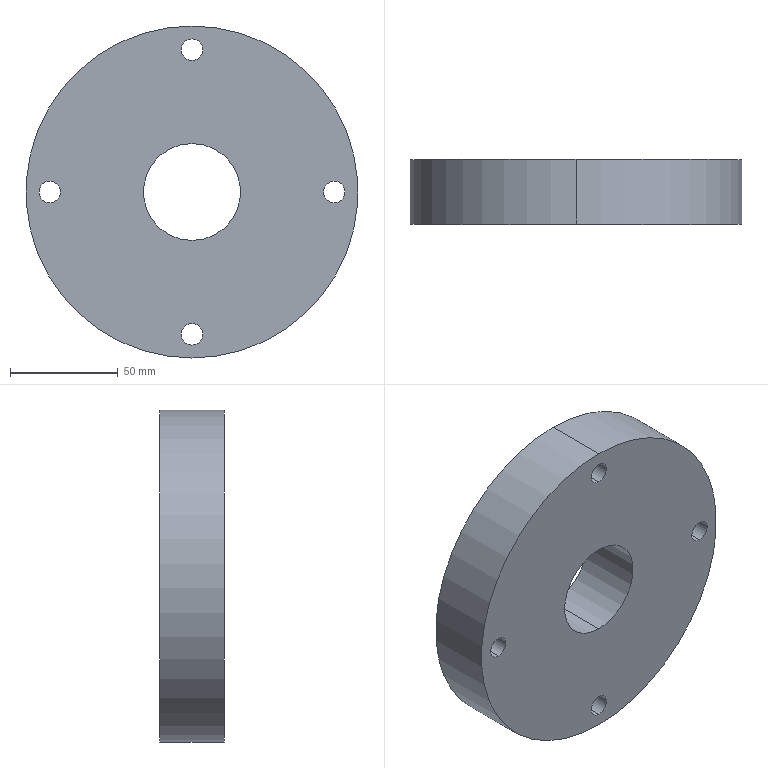Part | SolidWorks | features BaseBody 1 | 1 solid | 14 faces | box 154 x 30 x 154 mm | volume 501657 mm3 | cylinder 12 | plane 2 | commonest cylinder face diameters 10 x8 45 x2 154 x2
STEP:
#1=CARTESIAN_POINT('',(0.,30.,22.5));
#2=VERTEX_POINT('',#1);
#3=CARTESIAN_POINT('',(0.,30.,-22.5));
#4=VERTEX_POINT('',#3);
#5=CARTESIAN_POINT('',(0.,30.,0.));
#6=DIRECTION('',(0.,-1.,0.));
#7=DIRECTION('',(0.,0.,-1.));
#8=AXIS2_PLACEMENT_3D('',#5,#6,#7);
#9=CIRCLE('',#8,22.5);
#10=EDGE_CURVE('',#2,#4,#9,.T.);
#11=ORIENTED_EDGE('',*,*,#10,.F.);
#12=CARTESIAN_POINT('',(0.,0.,22.5));
#13=VERTEX_POINT('',#12);
#14=CARTESIAN_POINT('',(0.,30.,22.5));
#15=DIRECTION('',(0.,-1.,0.));
#16=VECTOR('',#15,1000.);
#17=LINE('',#14,#16);
#18=EDGE_CURVE('',#2,#13,#17,.T.);
#19=ORIENTED_EDGE('',*,*,#18,.T.);
#20=CARTESIAN_POINT('',(0.,0.,-22.5));
#21=VERTEX_POINT('',#20);
#22=CARTESIAN_POINT('',(0.,0.,0.));
#23=DIRECTION('',(0.,1.,0.));
#24=DIRECTION('',(0.,0.,-1.));
#25=AXIS2_PLACEMENT_3D('',#22,#23,#24);
#26=CIRCLE('',#25,22.5);
#27=EDGE_CURVE('',#21,#13,#26,.T.);
#28=ORIENTED_EDGE('',*,*,#27,.F.);
#29=CARTESIAN_POINT('',(0.,30.,-22.5));
#30=DIRECTION('',(0.,-1.,0.));
#31=VECTOR('',#30,1000.);
#32=LINE('',#29,#31);
#33=EDGE_CURVE('',#4,#21,#32,.T.);
#34=ORIENTED_EDGE('',*,*,#33,.F.);
#35=EDGE_LOOP('',(#11,#19,#28,#34));
#36=FACE_OUTER_BOUND('',#35,.T.);
#37=CARTESIAN_POINT('',(0.,30.,0.));
#38=DIRECTION('',(0.,-1.,0.));
#39=DIRECTION('',(0.,0.,-1.));
#40=AXIS2_PLACEMENT_3D('',#37,#38,#39);
#41=CYLINDRICAL_SURFACE('',#40,22.5);
#42=ADVANCED_FACE('',(#36),#41,.F.);
#43=CARTESIAN_POINT('',(0.,30.,77.));
#44=VERTEX_POINT('',#43);
#45=CARTESIAN_POINT('',(0.,30.,-77.));
#46=VERTEX_POINT('',#45);
#47=CARTESIAN_POINT('',(0.,30.,0.));
#48=DIRECTION('',(0.,1.,0.));
#49=DIRECTION('',(0.,0.,-1.));
#50=AXIS2_PLACEMENT_3D('',#47,#48,#49);
#51=CIRCLE('',#50,77.);
#52=EDGE_CURVE('',#44,#46,#51,.T.);
#53=ORIENTED_EDGE('',*,*,#52,.F.);
#54=CARTESIAN_POINT('',(0.,0.,77.));
#55=VERTEX_POINT('',#54);
#56=CARTESIAN_POINT('',(0.,30.,77.));
#57=DIRECTION('',(0.,-1.,0.));
#58=VECTOR('',#57,1000.);
#59=LINE('',#56,#58);
#60=EDGE_CURVE('',#44,#55,#59,.T.);
#61=ORIENTED_EDGE('',*,*,#60,.T.);
#62=CARTESIAN_POINT('',(0.,0.,-77.));
#63=VERTEX_POINT('',#62);
#64=CARTESIAN_POINT('',(0.,0.,0.));
#65=DIRECTION('',(0.,1.,0.));
#66=DIRECTION('',(0.,0.,-1.));
#67=AXIS2_PLACEMENT_3D('',#64,#65,#66);
#68=CIRCLE('',#67,77.);
#69=EDGE_CURVE('',#55,#63,#68,.T.);
#70=ORIENTED_EDGE('',*,*,#69,.T.);
#71=CARTESIAN_POINT('',(0.,30.,-77.));
#72=DIRECTION('',(0.,-1.,0.));
#73=VECTOR('',#72,1000.);
#74=LINE('',#71,#73);
#75=EDGE_CURVE('',#46,#63,#74,.T.);
#76=ORIENTED_EDGE('',*,*,#75,.F.);
#77=EDGE_LOOP('',(#53,#61,#70,#76));
#78=FACE_OUTER_BOUND('',#77,.T.);
#79=CARTESIAN_POINT('',(0.,30.,0.));
#80=DIRECTION('',(0.,-1.,0.));
#81=DIRECTION('',(0.,0.,-1.));
#82=AXIS2_PLACEMENT_3D('',#79,#80,#81);
#83=CYLINDRICAL_SURFACE('',#82,77.);
#84=ADVANCED_FACE('',(#78),#83,.T.);
#85=CARTESIAN_POINT('',(66.,30.,5.));
#86=VERTEX_POINT('',#85);
#87=CARTESIAN_POINT('',(66.,30.,-5.));
#88=VERTEX_POINT('',#87);
#89=CARTESIAN_POINT('',(66.,30.,0.));
#90=DIRECTION('',(0.,-1.,0.));
#91=DIRECTION('',(0.,0.,-1.));
#92=AXIS2_PLACEMENT_3D('',#89,#90,#91);
#93=CIRCLE('',#92,5.);
#94=EDGE_CURVE('',#86,#88,#93,.T.);
#95=ORIENTED_EDGE('',*,*,#94,.F.);
#96=CARTESIAN_POINT('',(66.,0.,5.));
#97=VERTEX_POINT('',#96);
#98=CARTESIAN_POINT('',(66.,30.,5.));
#99=DIRECTION('',(0.,-1.,0.));
#100=VECTOR('',#99,1000.);
#101=LINE('',#98,#100);
#102=EDGE_CURVE('',#86,#97,#101,.T.);
#103=ORIENTED_EDGE('',*,*,#102,.T.);
#104=CARTESIAN_POINT('',(66.,0.,-5.));
#105=VERTEX_POINT('',#104);
#106=CARTESIAN_POINT('',(66.,0.,0.));
#107=DIRECTION('',(0.,1.,0.));
#108=DIRECTION('',(0.,0.,-1.));
#109=AXIS2_PLACEMENT_3D('',#106,#107,#108);
#110=CIRCLE('',#109,5.);
#111=EDGE_CURVE('',#105,#97,#110,.T.);
#112=ORIENTED_EDGE('',*,*,#111,.F.);
#113=CARTESIAN_POINT('',(66.,30.,-5.));
#114=DIRECTION('',(0.,-1.,0.));
#115=VECTOR('',#114,1000.);
#116=LINE('',#113,#115);
#117=EDGE_CURVE('',#88,#105,#116,.T.);
#118=ORIENTED_EDGE('',*,*,#117,.F.);
#119=EDGE_LOOP('',(#95,#103,#112,#118));
#120=FACE_OUTER_BOUND('',#119,.T.);
#121=CARTESIAN_POINT('',(66.,30.,0.));
#122=DIRECTION('',(0.,-1.,0.));
#123=DIRECTION('',(0.,0.,-1.));
#124=AXIS2_PLACEMENT_3D('',#121,#122,#123);
#125=CYLINDRICAL_SURFACE('',#124,5.);
#126=ADVANCED_FACE('',(#120),#125,.F.);
#127=CARTESIAN_POINT('',(0.,30.,-61.));
#128=VERTEX_POINT('',#127);
#129=CARTESIAN_POINT('',(0.,30.,-71.));
#130=VERTEX_POINT('',#129);
#131=CARTESIAN_POINT('',(0.,30.,-66.));
#132=DIRECTION('',(0.,-1.,0.));
#133=DIRECTION('',(0.,0.,-1.));
#134=AXIS2_PLACEMENT_3D('',#131,#132,#133);
#135=CIRCLE('',#134,5.);
#136=EDGE_CURVE('',#128,#130,#135,.T.);
#137=ORIENTED_EDGE('',*,*,#136,.F.);
#138=CARTESIAN_POINT('',(0.,0.,-61.));
#139=VERTEX_POINT('',#138);
#140=CARTESIAN_POINT('',(0.,30.,-61.));
#141=DIRECTION('',(0.,-1.,0.));
#142=VECTOR('',#141,1000.);
#143=LINE('',#140,#142);
#144=EDGE_CURVE('',#128,#139,#143,.T.);
#145=ORIENTED_EDGE('',*,*,#144,.T.);
#146=CARTESIAN_POINT('',(0.,0.,-71.));
#147=VERTEX_POINT('',#146);
#148=CARTESIAN_POINT('',(0.,0.,-66.));
#149=DIRECTION('',(0.,1.,0.));
#150=DIRECTION('',(0.,0.,-1.));
#151=AXIS2_PLACEMENT_3D('',#148,#149,#150);
#152=CIRCLE('',#151,5.);
#153=EDGE_CURVE('',#147,#139,#152,.T.);
#154=ORIENTED_EDGE('',*,*,#153,.F.);
#155=CARTESIAN_POINT('',(0.,30.,-71.));
#156=DIRECTION('',(0.,-1.,0.));
#157=VECTOR('',#156,1000.);
#158=LINE('',#155,#157);
#159=EDGE_CURVE('',#130,#147,#158,.T.);
#160=ORIENTED_EDGE('',*,*,#159,.F.);
#161=EDGE_LOOP('',(#137,#145,#154,#160));
#162=FACE_OUTER_BOUND('',#161,.T.);
#163=CARTESIAN_POINT('',(0.,30.,-66.));
#164=DIRECTION('',(0.,-1.,0.));
#165=DIRECTION('',(0.,0.,-1.));
#166=AXIS2_PLACEMENT_3D('',#163,#164,#165);
#167=CYLINDRICAL_SURFACE('',#166,5.);
#168=ADVANCED_FACE('',(#162),#167,.F.);
#169=CARTESIAN_POINT('',(-66.,30.,5.));
#170=VERTEX_POINT('',#169);
#171=CARTESIAN_POINT('',(-66.,30.,-5.));
#172=VERTEX_POINT('',#171);
#173=CARTESIAN_POINT('',(-66.,30.,0.));
#174=DIRECTION('',(0.,-1.,0.));
#175=DIRECTION('',(0.,0.,-1.));
#176=AXIS2_PLACEMENT_3D('',#173,#174,#175);
#177=CIRCLE('',#176,5.);
#178=EDGE_CURVE('',#170,#172,#177,.T.);
#179=ORIENTED_EDGE('',*,*,#178,.F.);
#180=CARTESIAN_POINT('',(-66.,0.,5.));
#181=VERTEX_POINT('',#180);
#182=CARTESIAN_POINT('',(-66.,30.,5.));
#183=DIRECTION('',(0.,-1.,0.));
#184=VECTOR('',#183,1000.);
#185=LINE('',#182,#184);
#186=EDGE_CURVE('',#170,#181,#185,.T.);
#187=ORIENTED_EDGE('',*,*,#186,.T.);
#188=CARTESIAN_POINT('',(-66.,0.,-5.));
#189=VERTEX_POINT('',#188);
#190=CARTESIAN_POINT('',(-66.,0.,0.));
#191=DIRECTION('',(0.,1.,0.));
#192=DIRECTION('',(0.,0.,-1.));
#193=AXIS2_PLACEMENT_3D('',#190,#191,#192);
#194=CIRCLE('',#193,5.);
#195=EDGE_CURVE('',#189,#181,#194,.T.);
#196=ORIENTED_EDGE('',*,*,#195,.F.);
#197=CARTESIAN_POINT('',(-66.,30.,-5.));
#198=DIRECTION('',(0.,-1.,0.));
#199=VECTOR('',#198,1000.);
#200=LINE('',#197,#199);
#201=EDGE_CURVE('',#172,#189,#200,.T.);
#202=ORIENTED_EDGE('',*,*,#201,.F.);
#203=EDGE_LOOP('',(#179,#187,#196,#202));
#204=FACE_OUTER_BOUND('',#203,.T.);
#205=CARTESIAN_POINT('',(-66.,30.,0.));
#206=DIRECTION('',(0.,-1.,0.));
#207=DIRECTION('',(0.,0.,-1.));
#208=AXIS2_PLACEMENT_3D('',#205,#206,#207);
#209=CYLINDRICAL_SURFACE('',#208,5.);
#210=ADVANCED_FACE('',(#204),#209,.F.);
#211=CARTESIAN_POINT('',(0.,30.,71.));
#212=VERTEX_POINT('',#211);
#213=CARTESIAN_POINT('',(0.,30.,61.));
#214=VERTEX_POINT('',#213);
#215=CARTESIAN_POINT('',(0.,30.,66.));
#216=DIRECTION('',(0.,-1.,0.));
#217=DIRECTION('',(0.,0.,-1.));
#218=AXIS2_PLACEMENT_3D('',#215,#216,#217);
#219=CIRCLE('',#218,5.);
#220=EDGE_CURVE('',#212,#214,#219,.T.);
#221=ORIENTED_EDGE('',*,*,#220,.F.);
#222=CARTESIAN_POINT('',(0.,0.,71.));
#223=VERTEX_POINT('',#222);
#224=CARTESIAN_POINT('',(0.,30.,71.));
#225=DIRECTION('',(0.,-1.,0.));
#226=VECTOR('',#225,1000.);
#227=LINE('',#224,#226);
#228=EDGE_CURVE('',#212,#223,#227,.T.);
#229=ORIENTED_EDGE('',*,*,#228,.T.);
#230=CARTESIAN_POINT('',(0.,0.,61.));
#231=VERTEX_POINT('',#230);
#232=CARTESIAN_POINT('',(0.,0.,66.));
#233=DIRECTION('',(0.,1.,0.));
#234=DIRECTION('',(0.,0.,-1.));
#235=AXIS2_PLACEMENT_3D('',#232,#233,#234);
#236=CIRCLE('',#235,5.);
#237=EDGE_CURVE('',#231,#223,#236,.T.);
#238=ORIENTED_EDGE('',*,*,#237,.F.);
#239=CARTESIAN_POINT('',(0.,30.,61.));
#240=DIRECTION('',(0.,-1.,0.));
#241=VECTOR('',#240,1000.);
#242=LINE('',#239,#241);
#243=EDGE_CURVE('',#214,#231,#242,.T.);
#244=ORIENTED_EDGE('',*,*,#243,.F.);
#245=EDGE_LOOP('',(#221,#229,#238,#244));
#246=FACE_OUTER_BOUND('',#245,.T.);
#247=CARTESIAN_POINT('',(0.,30.,66.));
#248=DIRECTION('',(0.,-1.,0.));
#249=DIRECTION('',(0.,0.,-1.));
#250=AXIS2_PLACEMENT_3D('',#247,#248,#249);
#251=CYLINDRICAL_SURFACE('',#250,5.);
#252=ADVANCED_FACE('',(#246),#251,.F.);
#253=CARTESIAN_POINT('',(0.,30.,0.));
#254=DIRECTION('',(0.,-1.,0.));
#255=DIRECTION('',(0.,0.,-1.));
#256=AXIS2_PLACEMENT_3D('',#253,#254,#255);
#257=CIRCLE('',#256,22.5);
#258=EDGE_CURVE('',#4,#2,#257,.T.);
#259=ORIENTED_EDGE('',*,*,#258,.T.);
#260=ORIENTED_EDGE('',*,*,#10,.T.);
#261=EDGE_LOOP('',(#259,#260));
#262=FACE_BOUND('',#261,.T.);
#263=CARTESIAN_POINT('',(0.,30.,0.));
#264=DIRECTION('',(0.,1.,0.));
#265=DIRECTION('',(0.,0.,-1.));
#266=AXIS2_PLACEMENT_3D('',#263,#264,#265);
#267=CIRCLE('',#266,77.);
#268=EDGE_CURVE('',#46,#44,#267,.T.);
#269=ORIENTED_EDGE('',*,*,#268,.T.);
#270=ORIENTED_EDGE('',*,*,#52,.T.);
#271=EDGE_LOOP('',(#269,#270));
#272=FACE_OUTER_BOUND('',#271,.T.);
#273=CARTESIAN_POINT('',(66.,30.,0.));
#274=DIRECTION('',(0.,-1.,0.));
#275=DIRECTION('',(0.,0.,-1.));
#276=AXIS2_PLACEMENT_3D('',#273,#274,#275);
#277=CIRCLE('',#276,5.);
#278=EDGE_CURVE('',#88,#86,#277,.T.);
#279=ORIENTED_EDGE('',*,*,#278,.T.);
#280=ORIENTED_EDGE('',*,*,#94,.T.);
#281=EDGE_LOOP('',(#279,#280));
#282=FACE_BOUND('',#281,.T.);
#283=CARTESIAN_POINT('',(0.,30.,-66.));
#284=DIRECTION('',(0.,-1.,0.));
#285=DIRECTION('',(0.,0.,-1.));
#286=AXIS2_PLACEMENT_3D('',#283,#284,#285);
#287=CIRCLE('',#286,5.);
#288=EDGE_CURVE('',#130,#128,#287,.T.);
#289=ORIENTED_EDGE('',*,*,#288,.T.);
#290=ORIENTED_EDGE('',*,*,#136,.T.);
#291=EDGE_LOOP('',(#289,#290));
#292=FACE_BOUND('',#291,.T.);
#293=CARTESIAN_POINT('',(-66.,30.,0.));
#294=DIRECTION('',(0.,-1.,0.));
#295=DIRECTION('',(0.,0.,-1.));
#296=AXIS2_PLACEMENT_3D('',#293,#294,#295);
#297=CIRCLE('',#296,5.);
#298=EDGE_CURVE('',#172,#170,#297,.T.);
#299=ORIENTED_EDGE('',*,*,#298,.T.);
#300=ORIENTED_EDGE('',*,*,#178,.T.);
#301=EDGE_LOOP('',(#299,#300));
#302=FACE_BOUND('',#301,.T.);
#303=CARTESIAN_POINT('',(0.,30.,66.));
#304=DIRECTION('',(0.,-1.,0.));
#305=DIRECTION('',(0.,0.,-1.));
#306=AXIS2_PLACEMENT_3D('',#303,#304,#305);
#307=CIRCLE('',#306,5.);
#308=EDGE_CURVE('',#214,#212,#307,.T.);
#309=ORIENTED_EDGE('',*,*,#308,.T.);
#310=ORIENTED_EDGE('',*,*,#220,.T.);
#311=EDGE_LOOP('',(#309,#310));
#312=FACE_BOUND('',#311,.T.);
#313=CARTESIAN_POINT('',(0.,30.,0.));
#314=DIRECTION('',(0.,1.,0.));
#315=DIRECTION('',(0.,0.,1.));
#316=AXIS2_PLACEMENT_3D('',#313,#314,#315);
#317=PLANE('',#316);
#318=ADVANCED_FACE('',(#262,#272,#282,#292,#302,#312),#317,.T.);
#319=ORIENTED_EDGE('',*,*,#18,.F.);
#320=ORIENTED_EDGE('',*,*,#258,.F.);
#321=ORIENTED_EDGE('',*,*,#33,.T.);
#322=CARTESIAN_POINT('',(0.,0.,0.));
#323=DIRECTION('',(0.,1.,0.));
#324=DIRECTION('',(0.,0.,-1.));
#325=AXIS2_PLACEMENT_3D('',#322,#323,#324);
#326=CIRCLE('',#325,22.5);
#327=EDGE_CURVE('',#13,#21,#326,.T.);
#328=ORIENTED_EDGE('',*,*,#327,.F.);
#329=EDGE_LOOP('',(#319,#320,#321,#328));
#330=FACE_OUTER_BOUND('',#329,.T.);
#331=CARTESIAN_POINT('',(0.,30.,0.));
#332=DIRECTION('',(0.,-1.,0.));
#333=DIRECTION('',(0.,0.,-1.));
#334=AXIS2_PLACEMENT_3D('',#331,#332,#333);
#335=CYLINDRICAL_SURFACE('',#334,22.5);
#336=ADVANCED_FACE('',(#330),#335,.F.);
#337=ORIENTED_EDGE('',*,*,#60,.F.);
#338=ORIENTED_EDGE('',*,*,#268,.F.);
#339=ORIENTED_EDGE('',*,*,#75,.T.);
#340=CARTESIAN_POINT('',(0.,0.,0.));
#341=DIRECTION('',(0.,1.,0.));
#342=DIRECTION('',(0.,0.,-1.));
#343=AXIS2_PLACEMENT_3D('',#340,#341,#342);
#344=CIRCLE('',#343,77.);
#345=EDGE_CURVE('',#63,#55,#344,.T.);
#346=ORIENTED_EDGE('',*,*,#345,.T.);
#347=EDGE_LOOP('',(#337,#338,#339,#346));
#348=FACE_OUTER_BOUND('',#347,.T.);
#349=CARTESIAN_POINT('',(0.,30.,0.));
#350=DIRECTION('',(0.,-1.,0.));
#351=DIRECTION('',(0.,0.,-1.));
#352=AXIS2_PLACEMENT_3D('',#349,#350,#351);
#353=CYLINDRICAL_SURFACE('',#352,77.);
#354=ADVANCED_FACE('',(#348),#353,.T.);
#355=ORIENTED_EDGE('',*,*,#102,.F.);
#356=ORIENTED_EDGE('',*,*,#278,.F.);
#357=ORIENTED_EDGE('',*,*,#117,.T.);
#358=CARTESIAN_POINT('',(66.,0.,0.));
#359=DIRECTION('',(0.,1.,0.));
#360=DIRECTION('',(0.,0.,-1.));
#361=AXIS2_PLACEMENT_3D('',#358,#359,#360);
#362=CIRCLE('',#361,5.);
#363=EDGE_CURVE('',#97,#105,#362,.T.);
#364=ORIENTED_EDGE('',*,*,#363,.F.);
#365=EDGE_LOOP('',(#355,#356,#357,#364));
#366=FACE_OUTER_BOUND('',#365,.T.);
#367=CARTESIAN_POINT('',(66.,30.,0.));
#368=DIRECTION('',(0.,-1.,0.));
#369=DIRECTION('',(0.,0.,-1.));
#370=AXIS2_PLACEMENT_3D('',#367,#368,#369);
#371=CYLINDRICAL_SURFACE('',#370,5.);
#372=ADVANCED_FACE('',(#366),#371,.F.);
#373=ORIENTED_EDGE('',*,*,#144,.F.);
#374=ORIENTED_EDGE('',*,*,#288,.F.);
#375=ORIENTED_EDGE('',*,*,#159,.T.);
#376=CARTESIAN_POINT('',(0.,0.,-66.));
#377=DIRECTION('',(0.,1.,0.));
#378=DIRECTION('',(0.,0.,-1.));
#379=AXIS2_PLACEMENT_3D('',#376,#377,#378);
#380=CIRCLE('',#379,5.);
#381=EDGE_CURVE('',#139,#147,#380,.T.);
#382=ORIENTED_EDGE('',*,*,#381,.F.);
#383=EDGE_LOOP('',(#373,#374,#375,#382));
#384=FACE_OUTER_BOUND('',#383,.T.);
#385=CARTESIAN_POINT('',(0.,30.,-66.));
#386=DIRECTION('',(0.,-1.,0.));
#387=DIRECTION('',(0.,0.,-1.));
#388=AXIS2_PLACEMENT_3D('',#385,#386,#387);
#389=CYLINDRICAL_SURFACE('',#388,5.);
#390=ADVANCED_FACE('',(#384),#389,.F.);
#391=ORIENTED_EDGE('',*,*,#186,.F.);
#392=ORIENTED_EDGE('',*,*,#298,.F.);
#393=ORIENTED_EDGE('',*,*,#201,.T.);
#394=CARTESIAN_POINT('',(-66.,0.,0.));
#395=DIRECTION('',(0.,1.,0.));
#396=DIRECTION('',(0.,0.,-1.));
#397=AXIS2_PLACEMENT_3D('',#394,#395,#396);
#398=CIRCLE('',#397,5.);
#399=EDGE_CURVE('',#181,#189,#398,.T.);
#400=ORIENTED_EDGE('',*,*,#399,.F.);
#401=EDGE_LOOP('',(#391,#392,#393,#400));
#402=FACE_OUTER_BOUND('',#401,.T.);
#403=CARTESIAN_POINT('',(-66.,30.,0.));
#404=DIRECTION('',(0.,-1.,0.));
#405=DIRECTION('',(0.,0.,-1.));
#406=AXIS2_PLACEMENT_3D('',#403,#404,#405);
#407=CYLINDRICAL_SURFACE('',#406,5.);
#408=ADVANCED_FACE('',(#402),#407,.F.);
#409=ORIENTED_EDGE('',*,*,#228,.F.);
#410=ORIENTED_EDGE('',*,*,#308,.F.);
#411=ORIENTED_EDGE('',*,*,#243,.T.);
#412=CARTESIAN_POINT('',(0.,0.,66.));
#413=DIRECTION('',(0.,1.,0.));
#414=DIRECTION('',(0.,0.,-1.));
#415=AXIS2_PLACEMENT_3D('',#412,#413,#414);
#416=CIRCLE('',#415,5.);
#417=EDGE_CURVE('',#223,#231,#416,.T.);
#418=ORIENTED_EDGE('',*,*,#417,.F.);
#419=EDGE_LOOP('',(#409,#410,#411,#418));
#420=FACE_OUTER_BOUND('',#419,.T.);
#421=CARTESIAN_POINT('',(0.,30.,66.));
#422=DIRECTION('',(0.,-1.,0.));
#423=DIRECTION('',(0.,0.,-1.));
#424=AXIS2_PLACEMENT_3D('',#421,#422,#423);
#425=CYLINDRICAL_SURFACE('',#424,5.);
#426=ADVANCED_FACE('',(#420),#425,.F.);
#427=ORIENTED_EDGE('',*,*,#27,.T.);
#428=ORIENTED_EDGE('',*,*,#327,.T.);
#429=EDGE_LOOP('',(#427,#428));
#430=FACE_BOUND('',#429,.T.);
#431=ORIENTED_EDGE('',*,*,#345,.F.);
#432=ORIENTED_EDGE('',*,*,#69,.F.);
#433=EDGE_LOOP('',(#431,#432));
#434=FACE_OUTER_BOUND('',#433,.T.);
#435=ORIENTED_EDGE('',*,*,#111,.T.);
#436=ORIENTED_EDGE('',*,*,#363,.T.);
#437=EDGE_LOOP('',(#435,#436));
#438=FACE_BOUND('',#437,.T.);
#439=ORIENTED_EDGE('',*,*,#153,.T.);
#440=ORIENTED_EDGE('',*,*,#381,.T.);
#441=EDGE_LOOP('',(#439,#440));
#442=FACE_BOUND('',#441,.T.);
#443=ORIENTED_EDGE('',*,*,#195,.T.);
#444=ORIENTED_EDGE('',*,*,#399,.T.);
#445=EDGE_LOOP('',(#443,#444));
#446=FACE_BOUND('',#445,.T.);
#447=ORIENTED_EDGE('',*,*,#237,.T.);
#448=ORIENTED_EDGE('',*,*,#417,.T.);
#449=EDGE_LOOP('',(#447,#448));
#450=FACE_BOUND('',#449,.T.);
#451=CARTESIAN_POINT('',(0.,0.,0.));
#452=DIRECTION('',(0.,1.,0.));
#453=DIRECTION('',(0.,0.,1.));
#454=AXIS2_PLACEMENT_3D('',#451,#452,#453);
#455=PLANE('',#454);
#456=ADVANCED_FACE('',(#430,#434,#438,#442,#446,#450),#455,.F.);
#457=CLOSED_SHELL('',(#42,#84,#126,#168,#210,#252,#318,#336,#354,#372,#390,#408,#426,#456));
#458=MANIFOLD_SOLID_BREP('',#457);
#459=CARTESIAN_POINT('',(0.,0.,0.));
#460=DIRECTION('',(0.,0.,1.));
#461=DIRECTION('',(1.,0.,0.));
#462=AXIS2_PLACEMENT_3D('',#459,#460,#461);
#463=(LENGTH_UNIT()NAMED_UNIT(*)SI_UNIT(.MILLI.,.METRE.));
#464=UNCERTAINTY_MEASURE_WITH_UNIT(LENGTH_MEASURE(0.00001),#463,'','');
#465=(NAMED_UNIT(*)PLANE_ANGLE_UNIT()SI_UNIT($,.RADIAN.));
#466=(NAMED_UNIT(*)SI_UNIT($,.STERADIAN.)SOLID_ANGLE_UNIT());
#467=(GEOMETRIC_REPRESENTATION_CONTEXT(3)GLOBAL_UNCERTAINTY_ASSIGNED_CONTEXT((#464))GLOBAL_UNIT_ASSIGNED_CONTEXT((#463,#465,#466))REPRESENTATION_CONTEXT('',''));
#468=ADVANCED_BREP_SHAPE_REPRESENTATION('',(#458,#462),#467);